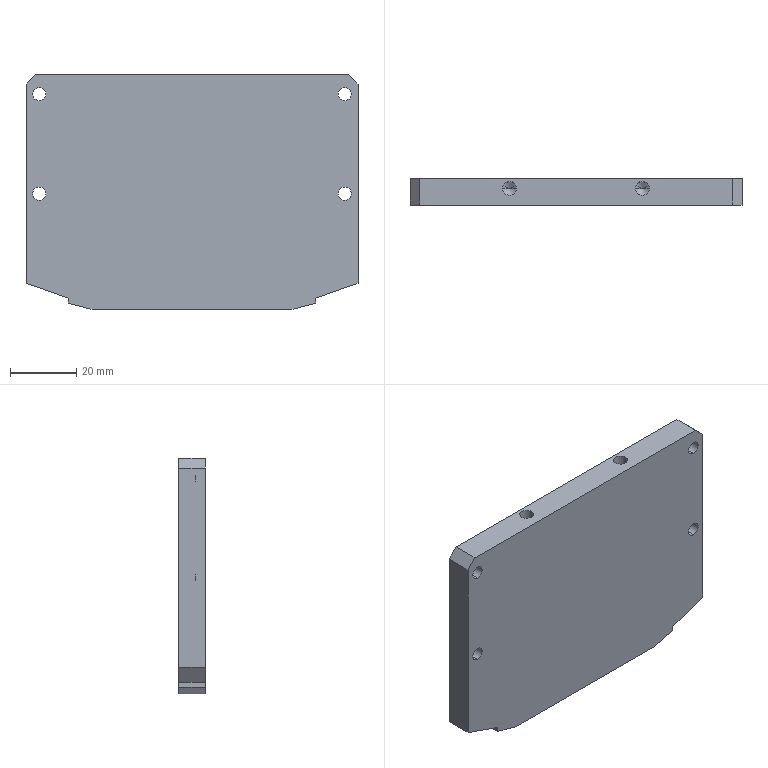Part | STEP file | lead screw Z-axis lower cover plate | 1 solid | 50 faces | box 100 x 8 x 71 mm | volume 53634 mm3 | cylinder 24 | plane 18 | cone 8 | commonest cylinder face diameters 4 x8 7.5 x8 3.3 x4 4.2 x4